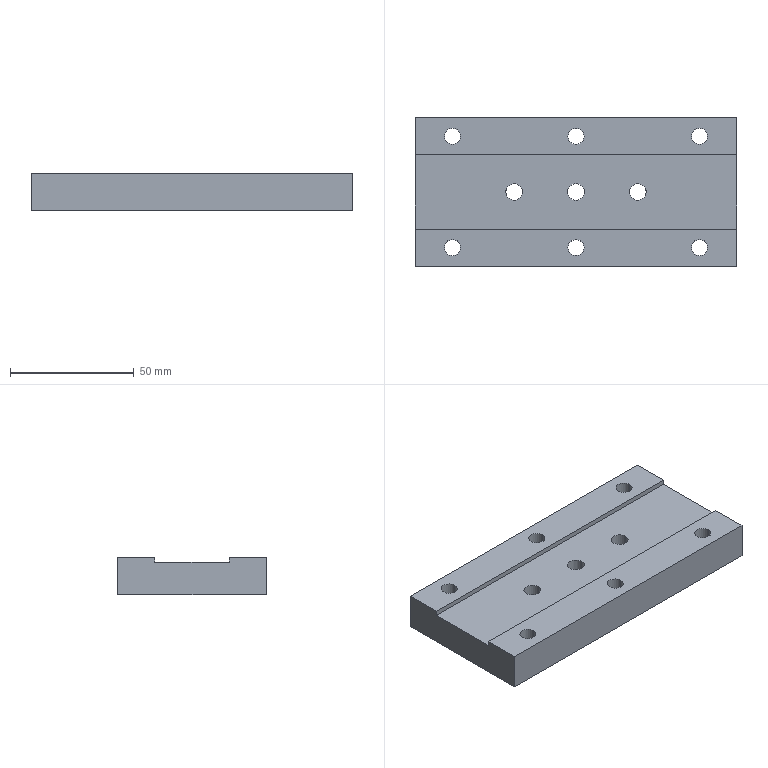Part | STEP file | A14 | 1 solid | 28 faces | box 130 x 60 x 15 mm | volume 104797 mm3 | cylinder 18 | plane 10 | commonest cylinder face diameters 6.5 x12 6.8 x6